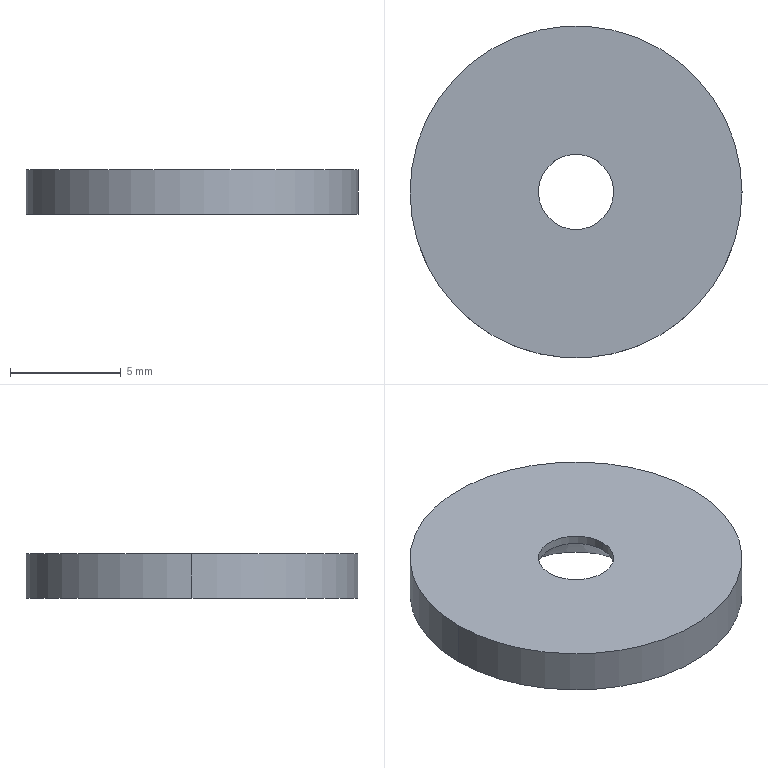Part | SolidWorks | features Extrusion 1, HoleWzd 1 | 1 solid | 8 faces | box 15 x 15 x 2 mm | volume 317.309 mm3 | cylinder 4 | cone 2 | plane 2 | commonest cylinder face diameters 3.4 x2 15 x2
STEP:
#1=CARTESIAN_POINT('',(1.7,0.,1.6));
#2=VERTEX_POINT('',#1);
#3=CARTESIAN_POINT('',(-1.7,0.,1.6));
#4=VERTEX_POINT('',#3);
#5=CARTESIAN_POINT('',(0.,0.,1.6));
#6=DIRECTION('',(0.,0.,-1.));
#7=DIRECTION('',(-1.,0.,0.));
#8=AXIS2_PLACEMENT_3D('',#5,#6,#7);
#9=CIRCLE('',#8,1.7);
#10=EDGE_CURVE('',#2,#4,#9,.T.);
#11=ORIENTED_EDGE('',*,*,#10,.F.);
#12=CARTESIAN_POINT('',(3.3,0.,0.));
#13=VERTEX_POINT('',#12);
#14=CARTESIAN_POINT('',(3.3,0.,0.));
#15=DIRECTION('',(0.7071,0.,-0.7071));
#16=VECTOR('',#15,1000.);
#17=LINE('',#14,#16);
#18=EDGE_CURVE('',#2,#13,#17,.T.);
#19=ORIENTED_EDGE('',*,*,#18,.T.);
#20=CARTESIAN_POINT('',(-3.3,0.,0.));
#21=VERTEX_POINT('',#20);
#22=CARTESIAN_POINT('',(0.,0.,0.));
#23=DIRECTION('',(0.,0.,-1.));
#24=DIRECTION('',(-1.,0.,0.));
#25=AXIS2_PLACEMENT_3D('',#22,#23,#24);
#26=CIRCLE('',#25,3.3);
#27=EDGE_CURVE('',#13,#21,#26,.T.);
#28=ORIENTED_EDGE('',*,*,#27,.T.);
#29=CARTESIAN_POINT('',(-3.3,0.,0.));
#30=DIRECTION('',(-0.7071,0.,-0.7071));
#31=VECTOR('',#30,1000.);
#32=LINE('',#29,#31);
#33=EDGE_CURVE('',#4,#21,#32,.T.);
#34=ORIENTED_EDGE('',*,*,#33,.F.);
#35=EDGE_LOOP('',(#11,#19,#28,#34));
#36=FACE_OUTER_BOUND('',#35,.T.);
#37=CARTESIAN_POINT('',(0.,0.,0.));
#38=DIRECTION('',(0.,0.,-1.));
#39=DIRECTION('',(-1.,0.,0.));
#40=AXIS2_PLACEMENT_3D('',#37,#38,#39);
#41=CONICAL_SURFACE('',#40,3.3,0.7854);
#42=ADVANCED_FACE('',(#36),#41,.F.);
#43=CARTESIAN_POINT('',(1.7,0.,2.));
#44=VERTEX_POINT('',#43);
#45=CARTESIAN_POINT('',(-1.7,0.,2.));
#46=VERTEX_POINT('',#45);
#47=CARTESIAN_POINT('',(0.,0.,2.));
#48=DIRECTION('',(0.,0.,-1.));
#49=DIRECTION('',(-1.,0.,0.));
#50=AXIS2_PLACEMENT_3D('',#47,#48,#49);
#51=CIRCLE('',#50,1.7);
#52=EDGE_CURVE('',#44,#46,#51,.T.);
#53=ORIENTED_EDGE('',*,*,#52,.F.);
#54=CARTESIAN_POINT('',(1.7,0.,0.));
#55=DIRECTION('',(0.,0.,-1.));
#56=VECTOR('',#55,1000.);
#57=LINE('',#54,#56);
#58=EDGE_CURVE('',#44,#2,#57,.T.);
#59=ORIENTED_EDGE('',*,*,#58,.T.);
#60=ORIENTED_EDGE('',*,*,#10,.T.);
#61=CARTESIAN_POINT('',(-1.7,0.,0.));
#62=DIRECTION('',(0.,0.,-1.));
#63=VECTOR('',#62,1000.);
#64=LINE('',#61,#63);
#65=EDGE_CURVE('',#46,#4,#64,.T.);
#66=ORIENTED_EDGE('',*,*,#65,.F.);
#67=EDGE_LOOP('',(#53,#59,#60,#66));
#68=FACE_OUTER_BOUND('',#67,.T.);
#69=CARTESIAN_POINT('',(0.,0.,0.));
#70=DIRECTION('',(0.,0.,-1.));
#71=DIRECTION('',(-1.,0.,0.));
#72=AXIS2_PLACEMENT_3D('',#69,#70,#71);
#73=CYLINDRICAL_SURFACE('',#72,1.7);
#74=ADVANCED_FACE('',(#68),#73,.F.);
#75=CARTESIAN_POINT('',(7.5,0.,2.));
#76=VERTEX_POINT('',#75);
#77=CARTESIAN_POINT('',(-7.5,0.,2.));
#78=VERTEX_POINT('',#77);
#79=CARTESIAN_POINT('',(0.,0.,2.));
#80=DIRECTION('',(0.,0.,1.));
#81=DIRECTION('',(1.,0.,0.));
#82=AXIS2_PLACEMENT_3D('',#79,#80,#81);
#83=CIRCLE('',#82,7.5);
#84=EDGE_CURVE('',#76,#78,#83,.T.);
#85=ORIENTED_EDGE('',*,*,#84,.F.);
#86=CARTESIAN_POINT('',(7.5,0.,0.));
#87=VERTEX_POINT('',#86);
#88=CARTESIAN_POINT('',(7.5,0.,2.));
#89=DIRECTION('',(0.,0.,-1.));
#90=VECTOR('',#89,1000.);
#91=LINE('',#88,#90);
#92=EDGE_CURVE('',#76,#87,#91,.T.);
#93=ORIENTED_EDGE('',*,*,#92,.T.);
#94=CARTESIAN_POINT('',(-7.5,0.,0.));
#95=VERTEX_POINT('',#94);
#96=CARTESIAN_POINT('',(0.,0.,0.));
#97=DIRECTION('',(0.,0.,1.));
#98=DIRECTION('',(1.,0.,0.));
#99=AXIS2_PLACEMENT_3D('',#96,#97,#98);
#100=CIRCLE('',#99,7.5);
#101=EDGE_CURVE('',#87,#95,#100,.T.);
#102=ORIENTED_EDGE('',*,*,#101,.T.);
#103=CARTESIAN_POINT('',(-7.5,0.,2.));
#104=DIRECTION('',(0.,0.,-1.));
#105=VECTOR('',#104,1000.);
#106=LINE('',#103,#105);
#107=EDGE_CURVE('',#78,#95,#106,.T.);
#108=ORIENTED_EDGE('',*,*,#107,.F.);
#109=EDGE_LOOP('',(#85,#93,#102,#108));
#110=FACE_OUTER_BOUND('',#109,.T.);
#111=CARTESIAN_POINT('',(0.,0.,2.));
#112=DIRECTION('',(0.,0.,-1.));
#113=DIRECTION('',(-1.,0.,0.));
#114=AXIS2_PLACEMENT_3D('',#111,#112,#113);
#115=CYLINDRICAL_SURFACE('',#114,7.5);
#116=ADVANCED_FACE('',(#110),#115,.T.);
#117=CARTESIAN_POINT('',(0.,0.,0.));
#118=DIRECTION('',(0.,0.,1.));
#119=DIRECTION('',(1.,0.,0.));
#120=AXIS2_PLACEMENT_3D('',#117,#118,#119);
#121=CIRCLE('',#120,7.5);
#122=EDGE_CURVE('',#95,#87,#121,.T.);
#123=ORIENTED_EDGE('',*,*,#122,.F.);
#124=ORIENTED_EDGE('',*,*,#101,.F.);
#125=EDGE_LOOP('',(#123,#124));
#126=FACE_OUTER_BOUND('',#125,.T.);
#127=CARTESIAN_POINT('',(0.,0.,0.));
#128=DIRECTION('',(0.,0.,-1.));
#129=DIRECTION('',(-1.,0.,0.));
#130=AXIS2_PLACEMENT_3D('',#127,#128,#129);
#131=CIRCLE('',#130,3.3);
#132=EDGE_CURVE('',#21,#13,#131,.T.);
#133=ORIENTED_EDGE('',*,*,#132,.F.);
#134=ORIENTED_EDGE('',*,*,#27,.F.);
#135=EDGE_LOOP('',(#133,#134));
#136=FACE_BOUND('',#135,.T.);
#137=CARTESIAN_POINT('',(0.,0.,0.));
#138=DIRECTION('',(0.,0.,1.));
#139=DIRECTION('',(1.,0.,0.));
#140=AXIS2_PLACEMENT_3D('',#137,#138,#139);
#141=PLANE('',#140);
#142=ADVANCED_FACE('',(#126,#136),#141,.F.);
#143=CARTESIAN_POINT('',(0.,0.,2.));
#144=DIRECTION('',(0.,0.,1.));
#145=DIRECTION('',(1.,0.,0.));
#146=AXIS2_PLACEMENT_3D('',#143,#144,#145);
#147=CIRCLE('',#146,7.5);
#148=EDGE_CURVE('',#78,#76,#147,.T.);
#149=ORIENTED_EDGE('',*,*,#148,.T.);
#150=ORIENTED_EDGE('',*,*,#84,.T.);
#151=EDGE_LOOP('',(#149,#150));
#152=FACE_OUTER_BOUND('',#151,.T.);
#153=CARTESIAN_POINT('',(0.,0.,2.));
#154=DIRECTION('',(0.,0.,-1.));
#155=DIRECTION('',(-1.,0.,0.));
#156=AXIS2_PLACEMENT_3D('',#153,#154,#155);
#157=CIRCLE('',#156,1.7);
#158=EDGE_CURVE('',#46,#44,#157,.T.);
#159=ORIENTED_EDGE('',*,*,#158,.T.);
#160=ORIENTED_EDGE('',*,*,#52,.T.);
#161=EDGE_LOOP('',(#159,#160));
#162=FACE_BOUND('',#161,.T.);
#163=CARTESIAN_POINT('',(0.,0.,2.));
#164=DIRECTION('',(0.,0.,1.));
#165=DIRECTION('',(1.,0.,0.));
#166=AXIS2_PLACEMENT_3D('',#163,#164,#165);
#167=PLANE('',#166);
#168=ADVANCED_FACE('',(#152,#162),#167,.T.);
#169=ORIENTED_EDGE('',*,*,#92,.F.);
#170=ORIENTED_EDGE('',*,*,#148,.F.);
#171=ORIENTED_EDGE('',*,*,#107,.T.);
#172=ORIENTED_EDGE('',*,*,#122,.T.);
#173=EDGE_LOOP('',(#169,#170,#171,#172));
#174=FACE_OUTER_BOUND('',#173,.T.);
#175=CARTESIAN_POINT('',(0.,0.,2.));
#176=DIRECTION('',(0.,0.,-1.));
#177=DIRECTION('',(-1.,0.,0.));
#178=AXIS2_PLACEMENT_3D('',#175,#176,#177);
#179=CYLINDRICAL_SURFACE('',#178,7.5);
#180=ADVANCED_FACE('',(#174),#179,.T.);
#181=ORIENTED_EDGE('',*,*,#58,.F.);
#182=ORIENTED_EDGE('',*,*,#158,.F.);
#183=ORIENTED_EDGE('',*,*,#65,.T.);
#184=CARTESIAN_POINT('',(0.,0.,1.6));
#185=DIRECTION('',(0.,0.,-1.));
#186=DIRECTION('',(-1.,0.,0.));
#187=AXIS2_PLACEMENT_3D('',#184,#185,#186);
#188=CIRCLE('',#187,1.7);
#189=EDGE_CURVE('',#4,#2,#188,.T.);
#190=ORIENTED_EDGE('',*,*,#189,.T.);
#191=EDGE_LOOP('',(#181,#182,#183,#190));
#192=FACE_OUTER_BOUND('',#191,.T.);
#193=CARTESIAN_POINT('',(0.,0.,0.));
#194=DIRECTION('',(0.,0.,-1.));
#195=DIRECTION('',(-1.,0.,0.));
#196=AXIS2_PLACEMENT_3D('',#193,#194,#195);
#197=CYLINDRICAL_SURFACE('',#196,1.7);
#198=ADVANCED_FACE('',(#192),#197,.F.);
#199=ORIENTED_EDGE('',*,*,#18,.F.);
#200=ORIENTED_EDGE('',*,*,#189,.F.);
#201=ORIENTED_EDGE('',*,*,#33,.T.);
#202=ORIENTED_EDGE('',*,*,#132,.T.);
#203=EDGE_LOOP('',(#199,#200,#201,#202));
#204=FACE_OUTER_BOUND('',#203,.T.);
#205=CARTESIAN_POINT('',(0.,0.,0.));
#206=DIRECTION('',(0.,0.,-1.));
#207=DIRECTION('',(-1.,0.,0.));
#208=AXIS2_PLACEMENT_3D('',#205,#206,#207);
#209=CONICAL_SURFACE('',#208,3.3,0.7854);
#210=ADVANCED_FACE('',(#204),#209,.F.);
#211=CLOSED_SHELL('',(#42,#74,#116,#142,#168,#180,#198,#210));
#212=MANIFOLD_SOLID_BREP('',#211);
#213=CARTESIAN_POINT('',(0.,0.,0.));
#214=DIRECTION('',(0.,0.,1.));
#215=DIRECTION('',(1.,0.,0.));
#216=AXIS2_PLACEMENT_3D('',#213,#214,#215);
#217=(LENGTH_UNIT()NAMED_UNIT(*)SI_UNIT(.MILLI.,.METRE.));
#218=UNCERTAINTY_MEASURE_WITH_UNIT(LENGTH_MEASURE(0.00001),#217,'','');
#219=(NAMED_UNIT(*)PLANE_ANGLE_UNIT()SI_UNIT($,.RADIAN.));
#220=(NAMED_UNIT(*)SI_UNIT($,.STERADIAN.)SOLID_ANGLE_UNIT());
#221=(GEOMETRIC_REPRESENTATION_CONTEXT(3)GLOBAL_UNCERTAINTY_ASSIGNED_CONTEXT((#218))GLOBAL_UNIT_ASSIGNED_CONTEXT((#217,#219,#220))REPRESENTATION_CONTEXT('',''));
#222=ADVANCED_BREP_SHAPE_REPRESENTATION('',(#212,#216),#221);